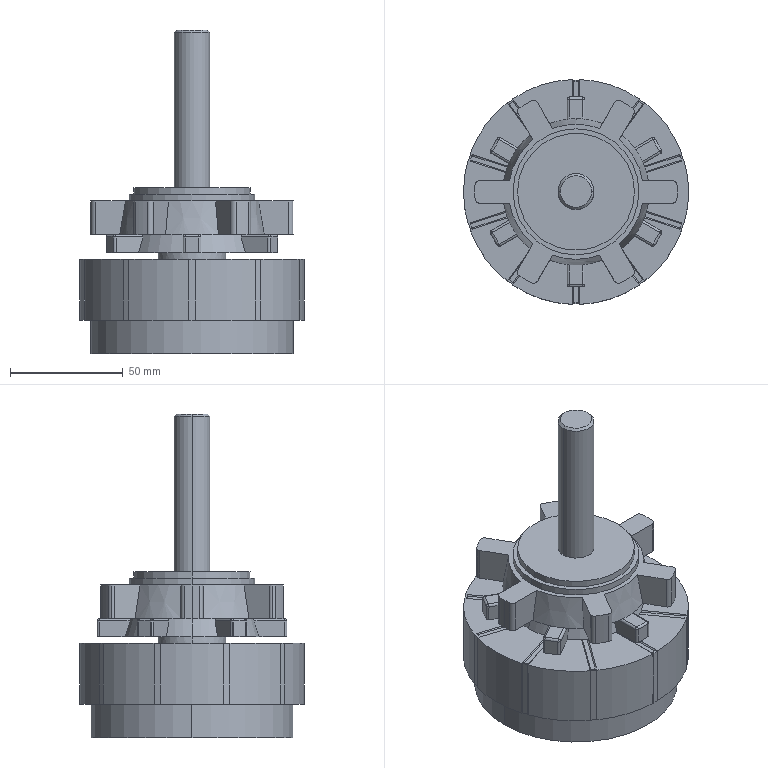Part | SolidWorks | features BaseBody 1 | 1 solid | 223 faces | box 100 x 99.955 x 144 mm | volume 420983 mm3 | plane 100 | cylinder 94 | cone 16 | sphere 13 | commonest cylinder face diameters 2 x32 1 x20 4 x14 100 x11 90 x9 16 x2